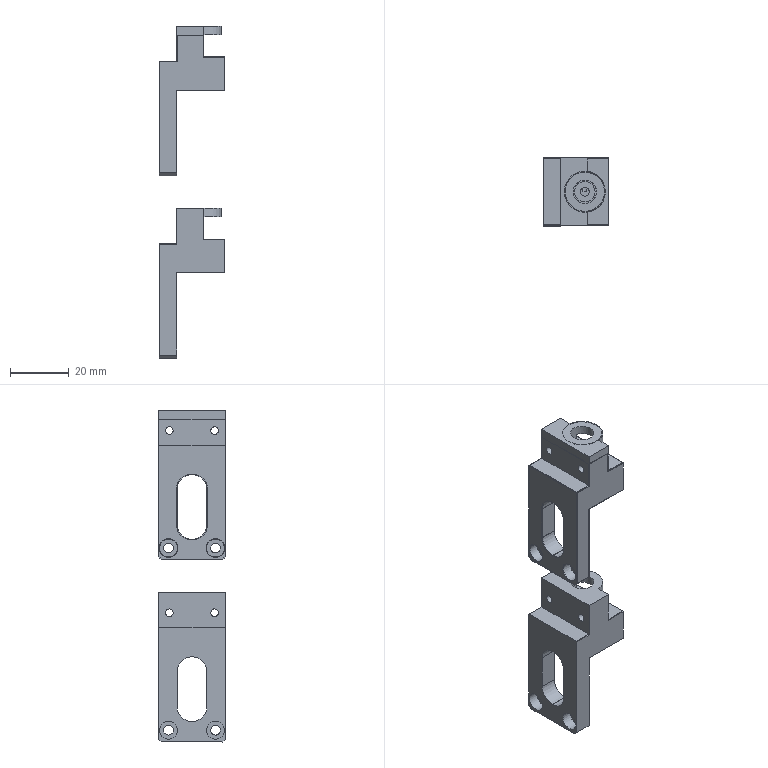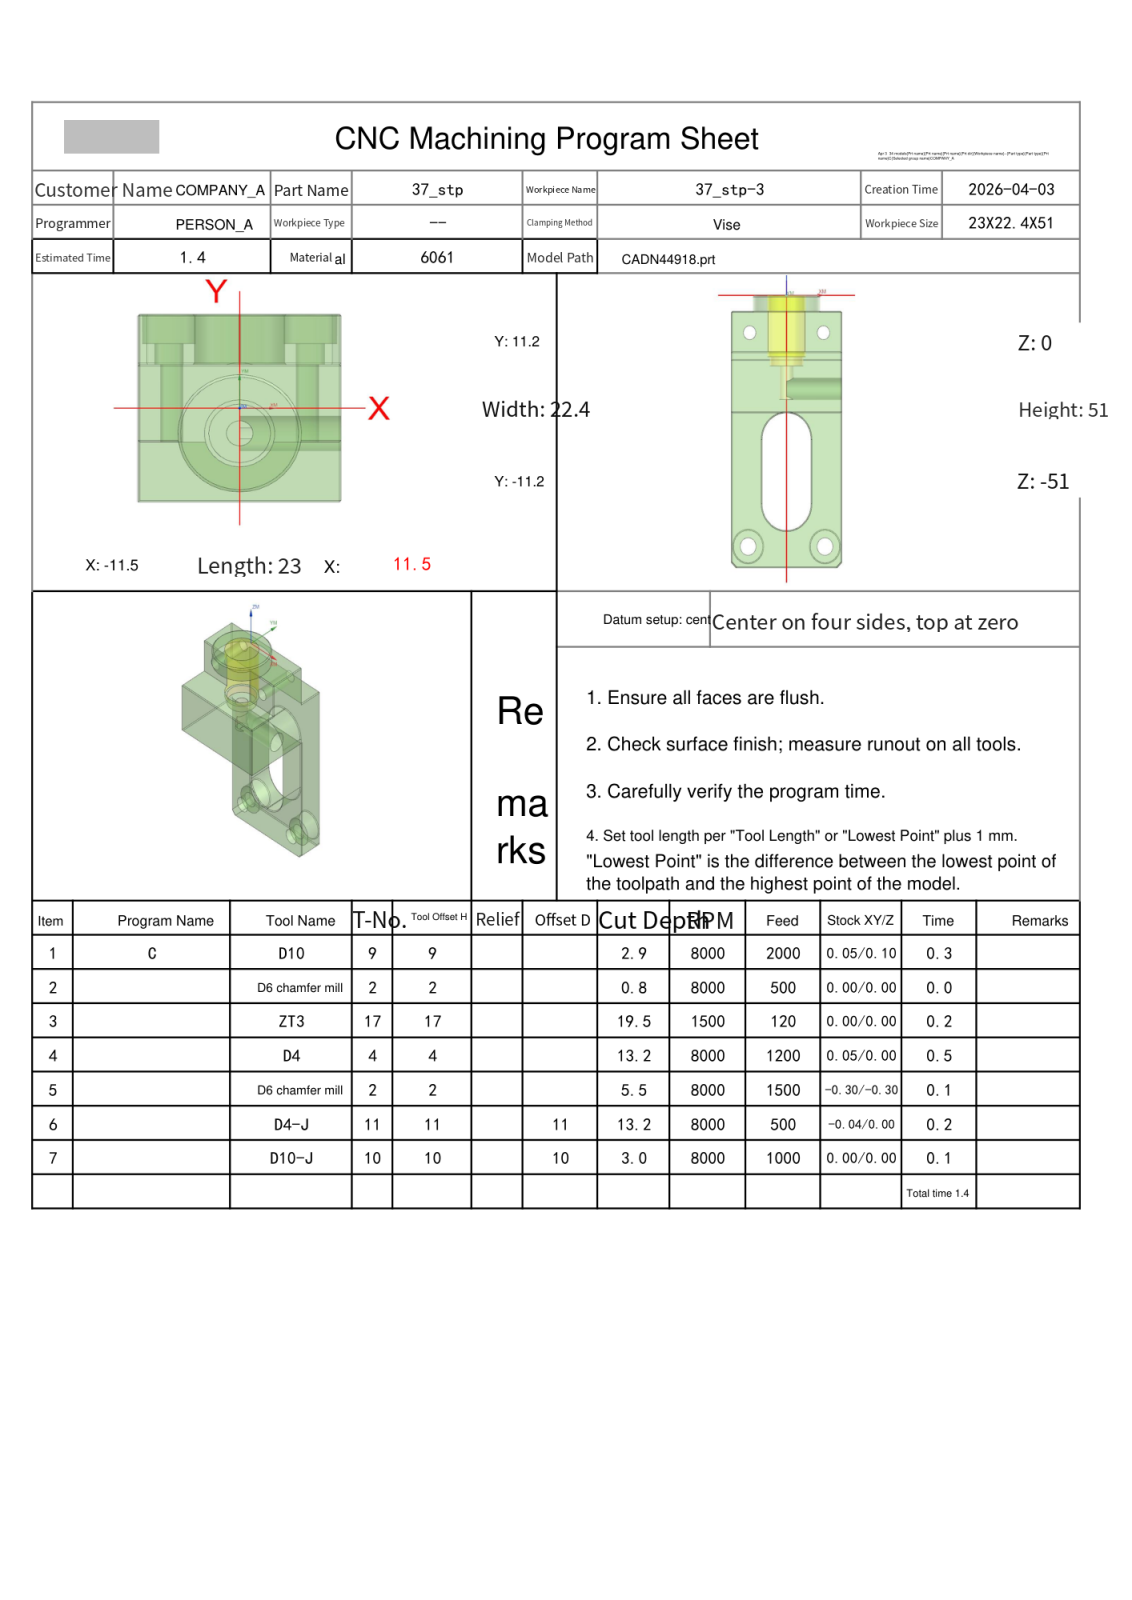NC program | NX | posted by the shop | part box 22.4 x 23 x 113 mm
Whole program:
%
O0001
(Machine time: 2.78 MIN)
(===Total Tool:6===)
(T9=D10     D=10.  R=0.   D-  H09 Z=-2.9  )
(T2=D6 chamfer mill   D=6.   R=0.   D-  H02 Z=-5.5  )
(T17=ZT3    D=3.   DR_a=118 D-  H17 Z=-19.5 )
(T4=D4      D=4.   R=0.   D-  H04 Z=-13.2 )
(T11=D4-J   D=4.   R=0.   D11 H11 Z=-13.2 )
(T10=D10-J  D=10.  R=0.   D10 H10 Z=-3.   )
G80 G90 G17 G49 G40
G91 G28 Z0
M01
N1 T09 M06
(D10  D=10. R=0. H=09 ce=0.05 di=0.10)
G00 G90 G54 X-10.037 Y-9.638 M03 S8000
G43 H09 Z20.
M08
Z1.
G01 X-10.469 Y-9.028 Z.961 F2000.
X-11.405 Y-6.981 Z.843
X-11.946 Y-4.795 Z.725
X-12.072 Y-2.548 Z.607
X-11.778 Y-.316 Z.489
X-11.075 Y1.823 Z.371
X-9.988 Y3.794 Z.253
X-8.554 Y5.53 Z.135
X-6.823 Y6.969 Z.017
X-5.354 Y7.829 Z-.072
X-3.162 Y8.659 Z-.195
X-.851 Y9.05 Z-.318
X0.0 Z-.363
G02 X12.05 Y-3. I0.0 J-12.05
X0.0 Y-15.05 I-12.05 J0.0
X-12.05 Y-3. I0.0 J12.05
X0.0 Y9.05 I12.05 J0.0
G01 X.384 Y9.044 Z-.383
X.768 Y9.026 Z-.403
X1.151 Y8.995 Z-.423
X1.533 Y8.952 Z-.443
X1.913 Y8.897 Z-.463
X2.292 Y8.83 Z-.483
X2.668 Y8.751 Z-.503
X3.041 Y8.66 Z-.524
X3.411 Y8.557 Z-.544
X3.778 Y8.442 Z-.564
X4.141 Y8.316 Z-.584
X4.5 Y8.178 Z-.604
X4.854 Y8.029 Z-.624
X5.203 Y7.869 Z-.644
X5.547 Y7.697 Z-.665
X5.885 Y7.515 Z-.685
X6.217 Y7.322 Z-.705
X6.543 Y7.119 Z-.725
G02 X12.05 Y-3. I-6.543 J-10.119
X0.0 Y-15.05 I-12.05 J0.0
X-12.05 Y-3. I0.0 J12.05
X0.0 Y9.05 I12.05 J0.0
G01 X.384 Y9.044 Z-.745
X.768 Y9.026 Z-.765
X1.151 Y8.995 Z-.785
X1.533 Y8.952 Z-.806
X1.913 Y8.897 Z-.826
X2.292 Y8.83 Z-.846
X2.668 Y8.751 Z-.866
X3.041 Y8.66 Z-.886
X3.411 Y8.557 Z-.906
X3.778 Y8.442 Z-.926
X4.141 Y8.316 Z-.947
X4.5 Y8.178 Z-.967
X4.854 Y8.029 Z-.987
X5.203 Y7.869 Z-1.007
X5.547 Y7.697 Z-1.027
X5.885 Y7.515 Z-1.047
X6.217 Y7.322 Z-1.067
X6.543 Y7.119 Z-1.088
G02 X12.05 Y-3. I-6.543 J-10.119
X0.0 Y-15.05 I-12.05 J0.0
X-12.05 Y-3. I0.0 J12.05
X0.0 Y9.05 I12.05 J0.0
G01 X.384 Y9.044 Z-1.108
X.768 Y9.026 Z-1.128
X1.151 Y8.995 Z-1.148
X1.533 Y8.952 Z-1.168
X1.913 Y8.897 Z-1.188
X2.292 Y8.83 Z-1.208
X2.668 Y8.751 Z-1.228
X3.041 Y8.66 Z-1.249
X3.411 Y8.557 Z-1.269
X3.778 Y8.442 Z-1.289
X4.141 Y8.316 Z-1.309
X4.5 Y8.178 Z-1.329
X4.854 Y8.029 Z-1.349
X5.203 Y7.869 Z-1.369
X5.547 Y7.697 Z-1.39
X5.885 Y7.515 Z-1.41
X6.217 Y7.322 Z-1.43
X6.543 Y7.119 Z-1.45
G02 X12.05 Y-3. I-6.543 J-10.119
X0.0 Y-15.05 I-12.05 J0.0
X-12.05 Y-3. I0.0 J12.05
X0.0 Y9.05 I12.05 J0.0
G01 X.384 Y9.044 Z-1.47
X.768 Y9.026 Z-1.49
X1.151 Y8.995 Z-1.51
X1.533 Y8.952 Z-1.531
X1.913 Y8.897 Z-1.551
X2.292 Y8.83 Z-1.571
X2.668 Y8.751 Z-1.591
X3.041 Y8.66 Z-1.611
X3.411 Y8.557 Z-1.631
X3.778 Y8.442 Z-1.651
X4.141 Y8.316 Z-1.672
X4.5 Y8.178 Z-1.692
X4.854 Y8.029 Z-1.712
X5.203 Y7.869 Z-1.732
X5.547 Y7.697 Z-1.752
X5.885 Y7.515 Z-1.772
X6.217 Y7.322 Z-1.792
X6.543 Y7.119 Z-1.813
G02 X12.05 Y-3. I-6.543 J-10.119
X0.0 Y-15.05 I-12.05 J0.0
X-12.05 Y-3. I0.0 J12.05
X0.0 Y9.05 I12.05 J0.0
G01 X.384 Y9.044 Z-1.833
X.768 Y9.026 Z-1.853
X1.151 Y8.995 Z-1.873
X1.533 Y8.952 Z-1.893
X1.913 Y8.897 Z-1.913
X2.292 Y8.83 Z-1.933
X2.668 Y8.751 Z-1.953
X3.041 Y8.66 Z-1.974
X3.411 Y8.557 Z-1.994
X3.778 Y8.442 Z-2.014
X4.141 Y8.316 Z-2.034
X4.5 Y8.178 Z-2.054
X4.854 Y8.029 Z-2.074
X5.203 Y7.869 Z-2.094
X5.547 Y7.697 Z-2.115
X5.885 Y7.515 Z-2.135
X6.217 Y7.322 Z-2.155
X6.543 Y7.119 Z-2.175
G02 X12.05 Y-3. I-6.543 J-10.119
X0.0 Y-15.05 I-12.05 J0.0
X-12.05 Y-3. I0.0 J12.05
X0.0 Y9.05 I12.05 J0.0
G01 X.384 Y9.044 Z-2.195
X.768 Y9.026 Z-2.215
X1.151 Y8.995 Z-2.235
X1.533 Y8.952 Z-2.256
X1.913 Y8.897 Z-2.276
X2.292 Y8.83 Z-2.296
X2.668 Y8.751 Z-2.316
X3.041 Y8.66 Z-2.336
X3.411 Y8.557 Z-2.356
X3.778 Y8.442 Z-2.376
X4.141 Y8.316 Z-2.397
X4.5 Y8.178 Z-2.417
X4.854 Y8.029 Z-2.437
X5.203 Y7.869 Z-2.457
X5.547 Y7.697 Z-2.477
X5.885 Y7.515 Z-2.497
X6.217 Y7.322 Z-2.517
X6.543 Y7.119 Z-2.538
G02 X12.05 Y-3. I-6.543 J-10.119
X0.0 Y-15.05 I-12.05 J0.0
X-12.05 Y-3. I0.0 J12.05
X0.0 Y9.05 I12.05 J0.0
G01 X.384 Y9.044 Z-2.558
X.768 Y9.026 Z-2.578
X1.151 Y8.995 Z-2.598
X1.533 Y8.952 Z-2.618
X1.913 Y8.897 Z-2.638
X2.292 Y8.83 Z-2.658
X2.668 Y8.751 Z-2.678
X3.041 Y8.66 Z-2.699
X3.411 Y8.557 Z-2.719
X3.778 Y8.442 Z-2.739
X4.141 Y8.316 Z-2.759
X4.5 Y8.178 Z-2.779
X4.854 Y8.029 Z-2.799
X5.203 Y7.869 Z-2.819
X5.547 Y7.697 Z-2.84
X5.885 Y7.515 Z-2.86
X6.217 Y7.322 Z-2.88
X6.543 Y7.119 Z-2.9
G02 X12.05 Y-3. I-6.543 J-10.119
X0.0 Y-15.05 I-12.05 J0.0
X-12.05 Y-3. I0.0 J12.05
X0.0 Y9.05 I12.05 J0.0
X6.543 Y7.119 I0.0 J-12.05
G01 Z-1.9
G00 Z20.
G91 G28 Z0.0
M05
M09
G91 G28 Z0.0
M01
N2 T02 M06
(D6 chamfer mill  D=6. R=0. H=02 ce=0.00 di=0.10)
G00 G90 G54 X0.0 Y-3. M03 S8000
G43 H02 Z20.
M08
G98 G81 X0.0 Y-3. Z-.8 R1. F500.
G80
G00 Z20.
G91 G28 Z0.0
M05
M09
G91 G28 Z0.0
M01
N3 T17 M06
(ZT3 D=3. DR_a=118 H=17)
G00 G90 G54 X0.0 Y-3. M03 S1500
G43 H17 Z20.
M08
G98 G83 X0.0 Y-3. Z-19.5 R1. F120. Q2.
G80
G00 Z20.
G91 G28 Z0.0
M05
M09
G91 G28 Z0.0
M01
N4 T04 M06
(D4  D=4. R=0. H=04 ce=0.05 di=0.00)
G00 G90 G54 X0.0 Y-3. M03 S8000
G43 H04 Z20.
M08
Z.5
G03 X-.975 Y-3.975 I0.0 J-.975 F1200.
X0.0 Y-4.95 I.975 J0.0
X0.0 Y-4.95 Z.2 I0.0 J1.95
X0.0 Y-4.95 Z-.1 I0.0 J1.95
X0.0 Y-4.95 Z-.4 I0.0 J1.95
X0.0 Y-4.95 Z-.7 I0.0 J1.95
X0.0 Y-4.95 Z-1. I0.0 J1.95
X0.0 Y-4.95 Z-1.3 I0.0 J1.95
X0.0 Y-4.95 Z-1.6 I0.0 J1.95
X0.0 Y-4.95 Z-1.9 I0.0 J1.95
X0.0 Y-4.95 Z-2.2 I0.0 J1.95
X0.0 Y-4.95 Z-2.5 I0.0 J1.95
X0.0 Y-4.95 Z-2.8 I0.0 J1.95
X0.0 Y-4.95 Z-3.1 I0.0 J1.95
X0.0 Y-4.95 Z-3.4 I0.0 J1.95
X0.0 Y-4.95 Z-3.7 I0.0 J1.95
X0.0 Y-4.95 Z-4. I0.0 J1.95
X0.0 Y-4.95 Z-4.3 I0.0 J1.95
X0.0 Y-4.95 Z-4.6 I0.0 J1.95
X0.0 Y-4.95 Z-4.9 I0.0 J1.95
X0.0 Y-4.95 Z-5.2 I0.0 J1.95
X0.0 Y-4.95 Z-5.5 I0.0 J1.95
X0.0 Y-4.95 Z-5.8 I0.0 J1.95
X0.0 Y-4.95 Z-6.1 I0.0 J1.95
X0.0 Y-4.95 Z-6.4 I0.0 J1.95
X0.0 Y-4.95 Z-6.7 I0.0 J1.95
X0.0 Y-4.95 Z-7. I0.0 J1.95
X0.0 Y-4.95 Z-7.3 I0.0 J1.95
X0.0 Y-4.95 Z-7.6 I0.0 J1.95
X0.0 Y-4.95 Z-7.9 I0.0 J1.95
X0.0 Y-4.95 Z-8.2 I0.0 J1.95
X0.0 Y-4.95 Z-8.5 I0.0 J1.95
X0.0 Y-4.95 Z-8.8 I0.0 J1.95
X0.0 Y-4.95 Z-9.1 I0.0 J1.95
X0.0 Y-4.95 Z-9.4 I0.0 J1.95
X0.0 Y-4.95 Z-9.7 I0.0 J1.95
X0.0 Y-4.95 Z-10. I0.0 J1.95
X0.0 Y-4.95 Z-10.3 I0.0 J1.95
X0.0 Y-4.95 Z-10.6 I0.0 J1.95
X0.0 Y-4.95 Z-10.9 I0.0 J1.95
X0.0 Y-4.95 Z-11.2 I0.0 J1.95
X0.0 Y-4.95 Z-11.5 I0.0 J1.95
X1.95 Y-3. I0.0 J1.95
X0.0 Y-1.05 I-1.95 J0.0
X-1.95 Y-3. I0.0 J-1.95
X0.0 Y-4.95 I1.95 J0.0
X.975 Y-3.975 I0.0 J.975
X0.0 Y-3. I-.975 J0.0
G00 Z20.
G00 G90 X0.0 Y-3. M03 S8000
Z20.
Z-11.
G03 X-.725 Y-3.725 I0.0 J-.725 F1200.
X0.0 Y-4.45 I.725 J0.0
X0.0 Y-4.45 Z-11.3 I0.0 J1.45
X0.0 Y-4.45 Z-11.6 I0.0 J1.45
X0.0 Y-4.45 Z-11.9 I0.0 J1.45
X0.0 Y-4.45 Z-12.2 I0.0 J1.45
X0.0 Y-4.45 Z-12.5 I0.0 J1.45
X0.0 Y-4.45 Z-12.8 I0.0 J1.45
X0.0 Y-4.45 Z-13.1 I0.0 J1.45
X1.256 Y-2.275 Z-13.2 I0.0 J1.45
X0.0 Y-1.55 I-1.256 J-.725
X-1.45 Y-3. I0.0 J-1.45
X0.0 Y-4.45 I1.45 J0.0
X1.45 Y-3. I0.0 J1.45
X1.256 Y-2.275 I-1.45 J0.0
X.628 Y-1.913 I-.628 J-.363
X-.097 Y-2.638 I0.0 J-.725
X0.0 Y-3. I.725 J0.0
G00 Z20.
G91 G28 Z0.0
M05
M09
G91 G28 Z0.0
M01
N5 T02 M06
(D6 chamfer mill  D=6. R=0. H=02 ce=-0.30 di=0.00)
G00 G90 G54 X2.099 Y-2.93 M03 S8000
G43 H02 Z20.
M08
Z-.7
G01 Z-1.2 F800.
X3. Y-2.9
G03 X0.0 Y.1 I-3. J0.0
X-3.1 Y-3. I0.0 J-3.1
X0.0 Y-6.1 I3.1 J0.0
X3.1 Y-3. I0.0 J3.1
X0.0 Y.1 I-3.1 J0.0
X-3. Y-2.9 I0.0 J-3.
G01 X-2.099 Y-2.93
Z-.7
G00 Z20.
G00 G90 X-.375 Y6.443 M03 S6500
Z20.
Z-1.354
G01 Z-2.5 F1500.
G03 X-.099 Y6.231 I1.351 J1.475
G01 X-.054 Y6.2
X0.0
G02 X9.2 Y-3. I0.0 J-9.2
X0.0 Y-12.2 I-9.2 J0.0
X-9.2 Y-3. I0.0 J9.2
X0.0 Y6.2 I9.2 J0.0
G01 X.054
X.099 Y6.231
G03 X.375 Y6.443 I-1.075 J1.687
G01 Z-1.354
G00 Z10.
X-9.625 Y-6.395
Z-1.538
G01 Z-5.5
X-9.682 Y-6.355
X-9.702 Y-6.35
X-11.3
G02 X-13.8 Y-3.85 I0.0 J2.5
G01 Y5.
G02 X-11.3 Y7.5 I2.5 J0.0
G01 X11.3
G02 X13.8 Y5. I0.0 J-2.5
G01 Y-3.85
G02 X11.3 Y-6.35 I-2.5 J0.0
G01 X9.702
X9.682 Y-6.355
X9.625 Y-6.395
Z-1.538
G00 Z20.
G91 G28 Z0.0
M05
M09
G91 G28 Z0.0
M01
N6 T11 M06
(D4-J  D=4. R=0. H=11 ce=0.00 di=0.00)
G00 G90 G54 X0.0 Y-3. M03 S8000
G43 H11 Z20.
M08
Z-11.
G41 D11
G01 X-.193 Y-3.052 F500.
G03 X-.737 Y-3.763 I.193 J-.711
X0.0 Y-4.5 I.737 J0.0
X.552 Y-1.605 Z-13.2 I0.0 J1.5
X0.0 Y-1.5 I-.552 J-1.395
X-1.5 Y-3. I0.0 J-1.5
X0.0 Y-4.5 I1.5 J0.0
X1.5 Y-3. I0.0 J1.5
X.552 Y-1.605 I-1.5 J0.0
X.281 Y-1.554 I-.271 J-.685
X-.456 Y-2.29 I0.0 J-.737
X-.16 Y-2.88 I.737 J0.0
G01 G40 X0.0 Y-3.
G00 Z20.
G00 G90 X-.6 Y-4.104 M03 S8000
Z10.
Z-2.333
G01 Z-3.833 F500.
G41 D11
Y-4.435
G03 X0.0 Y-5.035 I.6 J0.0
X2.035 Y-3. I0.0 J2.035
X0.0 Y-.965 I-2.035 J0.0
X-2.035 Y-3. I0.0 J-2.035
X0.0 Y-5.035 I2.035 J0.0
X.397 Y-4.996 I0.0 J2.035
X.88 Y-4.407 I-.117 J.588
G01 X.869 Y-4.29
X.843 Y-4.161
G40 X.804 Y-3.965
Z-2.333
G00 X-.6 Y-4.104
Z-6.167
G01 Z-7.667
G41 D11
Y-4.435
G03 X0.0 Y-5.035 I.6 J0.0
X2.035 Y-3. I0.0 J2.035
X0.0 Y-.965 I-2.035 J0.0
X-2.035 Y-3. I0.0 J-2.035
X0.0 Y-5.035 I2.035 J0.0
X.397 Y-4.996 I0.0 J2.035
X.88 Y-4.407 I-.117 J.588
G01 X.869 Y-4.29
X.843 Y-4.161
G40 X.804 Y-3.965
Z-6.167
G00 X-.6 Y-4.104
Z-10.
G01 Z-11.5
G41 D11
Y-4.435
G03 X0.0 Y-5.035 I.6 J0.0
X2.035 Y-3. I0.0 J2.035
X0.0 Y-.965 I-2.035 J0.0
X-2.035 Y-3. I0.0 J-2.035
X0.0 Y-5.035 I2.035 J0.0
X.397 Y-4.996 I0.0 J2.035
X.88 Y-4.407 I-.117 J.588
G01 X.869 Y-4.29
X.843 Y-4.161
G40 X.804 Y-3.965
Z-10.
G00 Z10.
G91 G28 Z0.0
M05
M09
G91 G28 Z0.0
M01
N7 T10 M06
(D10-J  D=10. R=0. H=10 ce=0.00 di=0.00)
G00 G90 G54 X-1.509 Y10.616 M03 S8000
G43 H10 Z5.
M08
Z-2.
G01 Z-3. F1000.
G41 D10
X-1.498 Y10.417
G03 X0.0 Y9. I1.498 J.083
G02 X12. Y-3. I0.0 J-12.
X0.0 Y-15. I-12. J0.0
X-12. Y-3. I0.0 J12.
X0.0 Y9. I12. J0.0
G03 X1.498 Y10.417 I0.0 J1.5
G01 G40 X1.509 Y10.616
Z-2.
G00 Z5.
M05
M09
G91 G28 Z0.0
G91 G28 Y0.0
M30
%